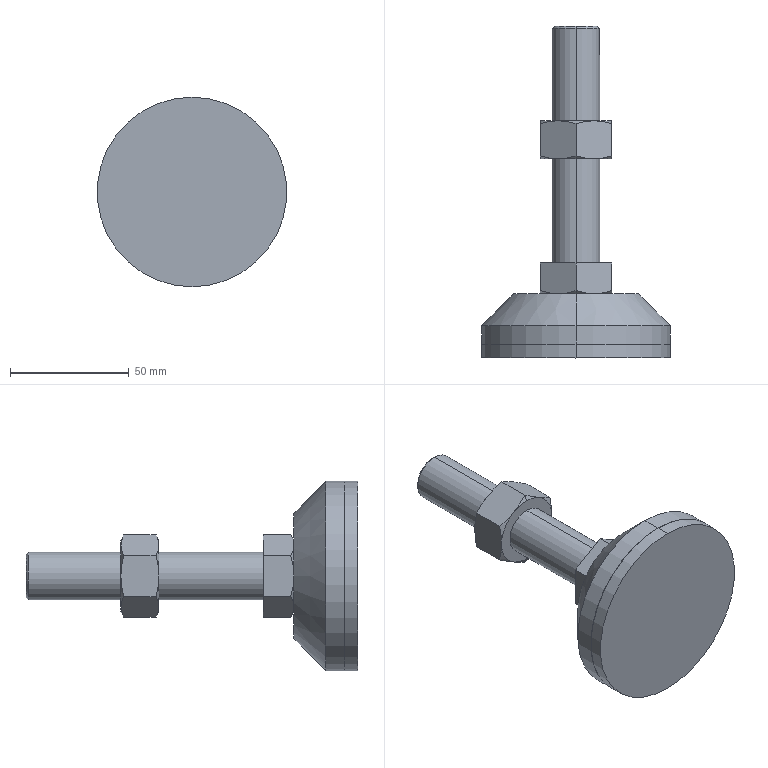Part | NX | features BREP 2 | 2 solids | 59 faces | box 80 x 140 x 80 mm | volume 165435 mm3 | cone 29 | plane 20 | cylinder 10 | commonest cylinder face diameters 80 x4 17.294 x2 20 x2 79.9 x2